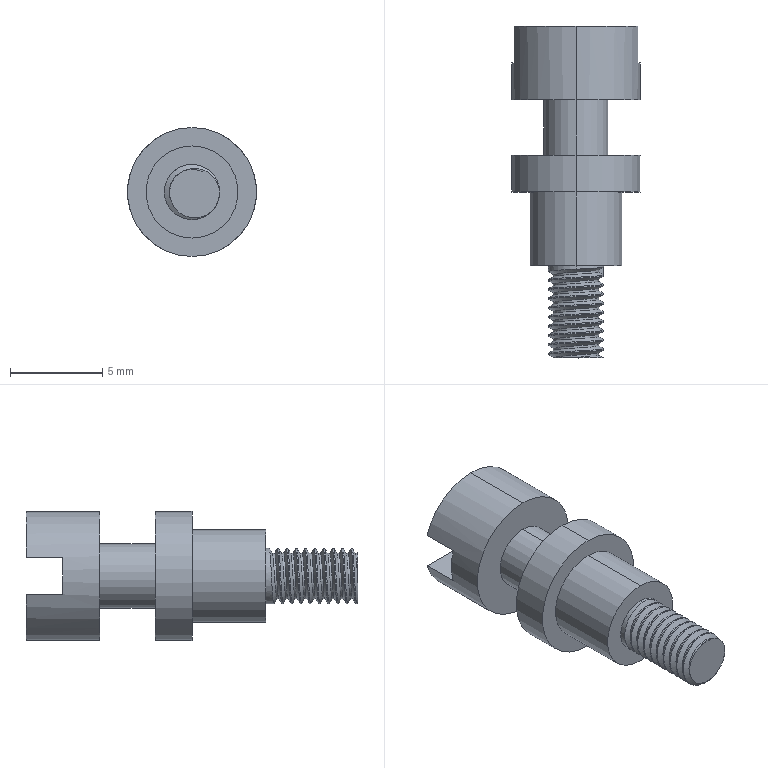Part | NX | features BREP 1 | 1 solid | 42 faces | box 7 x 18 x 7 mm | volume 340.606 mm3 | cylinder 29 | plane 11 | spline 2 | commonest cylinder face diameters 3 x20 7 x4 3.5 x2 5 x2 2.459 x1